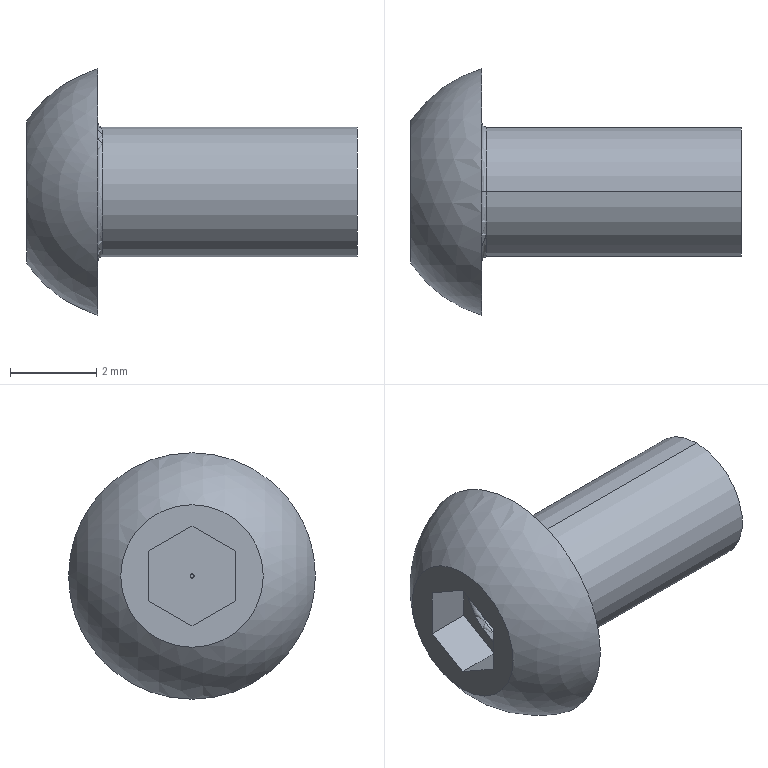Part | NX | features BREP 1 | 1 solid | 21 faces | box 7.65 x 5.7 x 5.7 mm | volume 68.684 mm3 | plane 10 | spline 6 | torus 2 | cylinder 2 | sphere 1 | commonest cylinder face diameters 3 x2
STEP:
#1=CARTESIAN_POINT('',(1.75,0.,1.5));
#2=VERTEX_POINT('',#1);
#3=CARTESIAN_POINT('',(1.75,0.,-1.5));
#4=VERTEX_POINT('',#3);
#5=CARTESIAN_POINT('',(1.75,0.,0.));
#6=DIRECTION('',(1.,0.,0.));
#7=DIRECTION('',(0.,0.,-1.));
#8=AXIS2_PLACEMENT_3D('',#5,#6,#7);
#9=CIRCLE('',#8,1.5);
#10=EDGE_CURVE('',#2,#4,#9,.T.);
#11=ORIENTED_EDGE('',*,*,#10,.F.);
#12=CARTESIAN_POINT('',(1.65,0.,1.6));
#13=VERTEX_POINT('',#12);
#14=CARTESIAN_POINT('',(1.75,0.,1.6));
#15=DIRECTION('',(0.,1.,0.));
#16=DIRECTION('',(0.,0.,1.));
#17=AXIS2_PLACEMENT_3D('',#14,#15,#16);
#18=CIRCLE('',#17,0.1);
#19=EDGE_CURVE('',#13,#2,#18,.F.);
#20=ORIENTED_EDGE('',*,*,#19,.F.);
#21=CARTESIAN_POINT('',(1.65,0.,-1.6));
#22=VERTEX_POINT('',#21);
#23=CARTESIAN_POINT('',(1.65,0.,0.));
#24=DIRECTION('',(-1.,0.,0.));
#25=DIRECTION('',(0.,0.,-1.));
#26=AXIS2_PLACEMENT_3D('',#23,#24,#25);
#27=CIRCLE('',#26,1.6);
#28=EDGE_CURVE('',#22,#13,#27,.T.);
#29=ORIENTED_EDGE('',*,*,#28,.F.);
#30=CARTESIAN_POINT('',(1.75,0.,-1.6));
#31=DIRECTION('',(0.,-1.,0.));
#32=DIRECTION('',(0.,0.,-1.));
#33=AXIS2_PLACEMENT_3D('',#30,#31,#32);
#34=CIRCLE('',#33,0.1);
#35=EDGE_CURVE('',#22,#4,#34,.F.);
#36=ORIENTED_EDGE('',*,*,#35,.T.);
#37=EDGE_LOOP('',(#11,#20,#29,#36));
#38=FACE_BOUND('',#37,.T.);
#39=CARTESIAN_POINT('',(1.75,0.,0.));
#40=DIRECTION('',(1.,0.,0.));
#41=DIRECTION('',(0.,0.,1.));
#42=AXIS2_PLACEMENT_3D('',#39,#40,#41);
#43=TOROIDAL_SURFACE('',#42,1.6,0.1);
#44=ADVANCED_FACE('',(#38),#43,.F.);
#45=CARTESIAN_POINT('',(7.65,0.,1.5));
#46=VERTEX_POINT('',#45);
#47=CARTESIAN_POINT('',(7.65,0.,-1.5));
#48=VERTEX_POINT('',#47);
#49=CARTESIAN_POINT('',(7.65,0.,0.));
#50=DIRECTION('',(-1.,0.,0.));
#51=DIRECTION('',(0.,0.,-1.));
#52=AXIS2_PLACEMENT_3D('',#49,#50,#51);
#53=CIRCLE('',#52,1.5);
#54=EDGE_CURVE('',#46,#48,#53,.T.);
#55=ORIENTED_EDGE('',*,*,#54,.T.);
#56=CARTESIAN_POINT('',(7.65,0.,-1.5));
#57=DIRECTION('',(-1.,0.,0.));
#58=VECTOR('',#57,1000.);
#59=LINE('',#56,#58);
#60=EDGE_CURVE('',#48,#4,#59,.T.);
#61=ORIENTED_EDGE('',*,*,#60,.T.);
#62=CARTESIAN_POINT('',(1.75,0.,0.));
#63=DIRECTION('',(1.,0.,0.));
#64=DIRECTION('',(0.,0.,-1.));
#65=AXIS2_PLACEMENT_3D('',#62,#63,#64);
#66=CIRCLE('',#65,1.5);
#67=EDGE_CURVE('',#4,#2,#66,.T.);
#68=ORIENTED_EDGE('',*,*,#67,.T.);
#69=CARTESIAN_POINT('',(7.65,0.,1.5));
#70=DIRECTION('',(-1.,0.,0.));
#71=VECTOR('',#70,1000.);
#72=LINE('',#69,#71);
#73=EDGE_CURVE('',#46,#2,#72,.T.);
#74=ORIENTED_EDGE('',*,*,#73,.F.);
#75=EDGE_LOOP('',(#55,#61,#68,#74));
#76=FACE_BOUND('',#75,.T.);
#77=CARTESIAN_POINT('',(7.65,0.,0.));
#78=DIRECTION('',(-1.,0.,0.));
#79=DIRECTION('',(0.,0.,-1.));
#80=AXIS2_PLACEMENT_3D('',#77,#78,#79);
#81=CYLINDRICAL_SURFACE('',#80,1.5);
#82=ADVANCED_FACE('',(#76),#81,.T.);
#83=CARTESIAN_POINT('',(1.65,2.85,0.));
#84=VERTEX_POINT('',#83);
#85=CARTESIAN_POINT('',(1.65,-2.85,0.));
#86=VERTEX_POINT('',#85);
#87=CARTESIAN_POINT('',(1.65,0.,0.));
#88=DIRECTION('',(1.,0.,0.));
#89=DIRECTION('',(0.,0.,-1.));
#90=AXIS2_PLACEMENT_3D('',#87,#88,#89);
#91=CIRCLE('',#90,2.85);
#92=EDGE_CURVE('',#84,#86,#91,.T.);
#93=ORIENTED_EDGE('',*,*,#92,.T.);
#94=CARTESIAN_POINT('',(1.65,0.,0.));
#95=DIRECTION('',(1.,0.,0.));
#96=DIRECTION('',(0.,0.,-1.));
#97=AXIS2_PLACEMENT_3D('',#94,#95,#96);
#98=CIRCLE('',#97,2.85);
#99=EDGE_CURVE('',#86,#84,#98,.T.);
#100=ORIENTED_EDGE('',*,*,#99,.T.);
#101=EDGE_LOOP('',(#93,#100));
#102=FACE_BOUND('',#101,.T.);
#103=ORIENTED_EDGE('',*,*,#28,.T.);
#104=CARTESIAN_POINT('',(1.65,0.,0.));
#105=DIRECTION('',(-1.,0.,0.));
#106=DIRECTION('',(0.,0.,-1.));
#107=AXIS2_PLACEMENT_3D('',#104,#105,#106);
#108=CIRCLE('',#107,1.6);
#109=EDGE_CURVE('',#13,#22,#108,.T.);
#110=ORIENTED_EDGE('',*,*,#109,.T.);
#111=EDGE_LOOP('',(#103,#110));
#112=FACE_BOUND('',#111,.T.);
#113=CARTESIAN_POINT('',(1.65,0.,0.));
#114=DIRECTION('',(1.,0.,0.));
#115=DIRECTION('',(0.,-1.,0.));
#116=AXIS2_PLACEMENT_3D('',#113,#114,#115);
#117=PLANE('',#116);
#118=ADVANCED_FACE('',(#102,#112),#117,.T.);
#119=ORIENTED_EDGE('',*,*,#92,.F.);
#120=ORIENTED_EDGE('',*,*,#99,.F.);
#121=EDGE_LOOP('',(#119,#120));
#122=FACE_BOUND('',#121,.T.);
#123=CARTESIAN_POINT('',(0.,1.65,0.));
#124=VERTEX_POINT('',#123);
#125=CARTESIAN_POINT('',(0.,-1.65,0.));
#126=VERTEX_POINT('',#125);
#127=CARTESIAN_POINT('',(0.,0.,0.));
#128=DIRECTION('',(1.,0.,0.));
#129=DIRECTION('',(0.,0.,-1.));
#130=AXIS2_PLACEMENT_3D('',#127,#128,#129);
#131=CIRCLE('',#130,1.65);
#132=EDGE_CURVE('',#124,#126,#131,.T.);
#133=ORIENTED_EDGE('',*,*,#132,.T.);
#134=CARTESIAN_POINT('',(0.,0.,0.));
#135=DIRECTION('',(1.,0.,0.));
#136=DIRECTION('',(0.,0.,-1.));
#137=AXIS2_PLACEMENT_3D('',#134,#135,#136);
#138=CIRCLE('',#137,1.65);
#139=EDGE_CURVE('',#126,#124,#138,.T.);
#140=ORIENTED_EDGE('',*,*,#139,.T.);
#141=EDGE_LOOP('',(#133,#140));
#142=FACE_BOUND('',#141,.T.);
#143=CARTESIAN_POINT('',(2.461,0.,0.));
#144=DIRECTION('',(0.,1.,0.));
#145=DIRECTION('',(-0.2585,0.,-0.966));
#146=AXIS2_PLACEMENT_3D('',#143,#144,#145);
#147=SPHERICAL_SURFACE('',#146,2.963);
#148=ADVANCED_FACE('',(#122,#142),#147,.T.);
#149=ORIENTED_EDGE('',*,*,#132,.F.);
#150=ORIENTED_EDGE('',*,*,#139,.F.);
#151=EDGE_LOOP('',(#149,#150));
#152=FACE_BOUND('',#151,.T.);
#153=CARTESIAN_POINT('',(0.,1.,-0.5774));
#154=VERTEX_POINT('',#153);
#155=CARTESIAN_POINT('',(0.,0.,-1.155));
#156=VERTEX_POINT('',#155);
#157=CARTESIAN_POINT('',(0.,1.,-0.5774));
#158=DIRECTION('',(0.,-0.866,-0.5));
#159=VECTOR('',#158,1000.);
#160=LINE('',#157,#159);
#161=EDGE_CURVE('',#154,#156,#160,.T.);
#162=ORIENTED_EDGE('',*,*,#161,.F.);
#163=CARTESIAN_POINT('',(0.,1.,0.5774));
#164=VERTEX_POINT('',#163);
#165=CARTESIAN_POINT('',(0.,1.,0.));
#166=DIRECTION('',(0.,0.,-1.));
#167=VECTOR('',#166,1000.);
#168=LINE('',#165,#167);
#169=EDGE_CURVE('',#164,#154,#168,.T.);
#170=ORIENTED_EDGE('',*,*,#169,.F.);
#171=CARTESIAN_POINT('',(0.,0.,1.155));
#172=VERTEX_POINT('',#171);
#173=CARTESIAN_POINT('',(0.,0.,1.155));
#174=DIRECTION('',(0.,0.866,-0.5));
#175=VECTOR('',#174,1000.);
#176=LINE('',#173,#175);
#177=EDGE_CURVE('',#172,#164,#176,.T.);
#178=ORIENTED_EDGE('',*,*,#177,.F.);
#179=CARTESIAN_POINT('',(0.,-1.,0.5774));
#180=VERTEX_POINT('',#179);
#181=CARTESIAN_POINT('',(0.,-1.,0.5774));
#182=DIRECTION('',(0.,0.866,0.5));
#183=VECTOR('',#182,1000.);
#184=LINE('',#181,#183);
#185=EDGE_CURVE('',#180,#172,#184,.T.);
#186=ORIENTED_EDGE('',*,*,#185,.F.);
#187=CARTESIAN_POINT('',(0.,-1.,-0.5774));
#188=VERTEX_POINT('',#187);
#189=CARTESIAN_POINT('',(0.,-1.,0.));
#190=DIRECTION('',(0.,0.,1.));
#191=VECTOR('',#190,1000.);
#192=LINE('',#189,#191);
#193=EDGE_CURVE('',#188,#180,#192,.T.);
#194=ORIENTED_EDGE('',*,*,#193,.F.);
#195=CARTESIAN_POINT('',(0.,0.,-1.155));
#196=DIRECTION('',(0.,-0.866,0.5));
#197=VECTOR('',#196,1000.);
#198=LINE('',#195,#197);
#199=EDGE_CURVE('',#156,#188,#198,.T.);
#200=ORIENTED_EDGE('',*,*,#199,.F.);
#201=EDGE_LOOP('',(#162,#170,#178,#186,#194,#200));
#202=FACE_BOUND('',#201,.T.);
#203=CARTESIAN_POINT('',(0.,0.,0.));
#204=DIRECTION('',(1.,0.,0.));
#205=DIRECTION('',(0.,-1.,0.));
#206=AXIS2_PLACEMENT_3D('',#203,#204,#205);
#207=PLANE('',#206);
#208=ADVANCED_FACE('',(#152,#202),#207,.F.);
#209=CARTESIAN_POINT('',(1.04,-1.,-0.5774));
#210=VERTEX_POINT('',#209);
#211=CARTESIAN_POINT('',(1.04,0.,-1.155));
#212=VERTEX_POINT('',#211);
#213=CARTESIAN_POINT('',(1.04,-1.,-0.5774));
#214=DIRECTION('',(0.,0.866,-0.5));
#215=VECTOR('',#214,1000.);
#216=LINE('',#213,#215);
#217=EDGE_CURVE('',#210,#212,#216,.T.);
#218=ORIENTED_EDGE('',*,*,#217,.T.);
#219=CARTESIAN_POINT('',(1.04,0.,-1.155));
#220=DIRECTION('',(-1.,0.,0.));
#221=VECTOR('',#220,1000.);
#222=LINE('',#219,#221);
#223=EDGE_CURVE('',#212,#156,#222,.T.);
#224=ORIENTED_EDGE('',*,*,#223,.T.);
#225=ORIENTED_EDGE('',*,*,#199,.T.);
#226=CARTESIAN_POINT('',(1.04,-1.,-0.5774));
#227=DIRECTION('',(1.,0.,0.));
#228=VECTOR('',#227,1000.);
#229=LINE('',#226,#228);
#230=EDGE_CURVE('',#188,#210,#229,.T.);
#231=ORIENTED_EDGE('',*,*,#230,.T.);
#232=EDGE_LOOP('',(#218,#224,#225,#231));
#233=FACE_BOUND('',#232,.T.);
#234=CARTESIAN_POINT('',(1.04,-1.,-0.5774));
#235=DIRECTION('',(0.,0.5,0.866));
#236=DIRECTION('',(-1.,0.,0.));
#237=AXIS2_PLACEMENT_3D('',#234,#235,#236);
#238=PLANE('',#237);
#239=ADVANCED_FACE('',(#233),#238,.T.);
#240=CARTESIAN_POINT('',(1.04,1.,-0.5774));
#241=VERTEX_POINT('',#240);
#242=CARTESIAN_POINT('',(1.04,0.,-1.155));
#243=DIRECTION('',(0.,0.866,0.5));
#244=VECTOR('',#243,1000.);
#245=LINE('',#242,#244);
#246=EDGE_CURVE('',#212,#241,#245,.T.);
#247=ORIENTED_EDGE('',*,*,#246,.T.);
#248=CARTESIAN_POINT('',(1.04,1.,-0.5774));
#249=DIRECTION('',(-1.,0.,0.));
#250=VECTOR('',#249,1000.);
#251=LINE('',#248,#250);
#252=EDGE_CURVE('',#241,#154,#251,.T.);
#253=ORIENTED_EDGE('',*,*,#252,.T.);
#254=ORIENTED_EDGE('',*,*,#161,.T.);
#255=ORIENTED_EDGE('',*,*,#223,.F.);
#256=EDGE_LOOP('',(#247,#253,#254,#255));
#257=FACE_BOUND('',#256,.T.);
#258=CARTESIAN_POINT('',(1.04,0.,-1.155));
#259=DIRECTION('',(0.,-0.5,0.866));
#260=DIRECTION('',(1.,0.,0.));
#261=AXIS2_PLACEMENT_3D('',#258,#259,#260);
#262=PLANE('',#261);
#263=ADVANCED_FACE('',(#257),#262,.T.);
#264=CARTESIAN_POINT('',(1.04,1.,0.5774));
#265=VERTEX_POINT('',#264);
#266=CARTESIAN_POINT('',(1.04,1.,-0.5774));
#267=DIRECTION('',(0.,0.,1.));
#268=VECTOR('',#267,1000.);
#269=LINE('',#266,#268);
#270=EDGE_CURVE('',#241,#265,#269,.T.);
#271=ORIENTED_EDGE('',*,*,#270,.T.);
#272=CARTESIAN_POINT('',(1.04,1.,0.5774));
#273=DIRECTION('',(-1.,0.,0.));
#274=VECTOR('',#273,1000.);
#275=LINE('',#272,#274);
#276=EDGE_CURVE('',#265,#164,#275,.T.);
#277=ORIENTED_EDGE('',*,*,#276,.T.);
#278=ORIENTED_EDGE('',*,*,#169,.T.);
#279=ORIENTED_EDGE('',*,*,#252,.F.);
#280=EDGE_LOOP('',(#271,#277,#278,#279));
#281=FACE_BOUND('',#280,.T.);
#282=CARTESIAN_POINT('',(1.04,1.,-0.5774));
#283=DIRECTION('',(0.,-1.,0.));
#284=DIRECTION('',(1.,0.,0.));
#285=AXIS2_PLACEMENT_3D('',#282,#283,#284);
#286=PLANE('',#285);
#287=ADVANCED_FACE('',(#281),#286,.T.);
#288=CARTESIAN_POINT('',(1.04,0.,1.155));
#289=VERTEX_POINT('',#288);
#290=CARTESIAN_POINT('',(1.04,1.,0.5774));
#291=DIRECTION('',(0.,-0.866,0.5));
#292=VECTOR('',#291,1000.);
#293=LINE('',#290,#292);
#294=EDGE_CURVE('',#265,#289,#293,.T.);
#295=ORIENTED_EDGE('',*,*,#294,.T.);
#296=CARTESIAN_POINT('',(1.04,0.,1.155));
#297=DIRECTION('',(-1.,0.,0.));
#298=VECTOR('',#297,1000.);
#299=LINE('',#296,#298);
#300=EDGE_CURVE('',#289,#172,#299,.T.);
#301=ORIENTED_EDGE('',*,*,#300,.T.);
#302=ORIENTED_EDGE('',*,*,#177,.T.);
#303=ORIENTED_EDGE('',*,*,#276,.F.);
#304=EDGE_LOOP('',(#295,#301,#302,#303));
#305=FACE_BOUND('',#304,.T.);
#306=CARTESIAN_POINT('',(1.04,1.,0.5774));
#307=DIRECTION('',(0.,-0.5,-0.866));
#308=DIRECTION('',(0.,0.866,-0.5));
#309=AXIS2_PLACEMENT_3D('',#306,#307,#308);
#310=PLANE('',#309);
#311=ADVANCED_FACE('',(#305),#310,.T.);
#312=CARTESIAN_POINT('',(1.04,-1.,0.5774));
#313=VERTEX_POINT('',#312);
#314=CARTESIAN_POINT('',(1.04,0.,1.155));
#315=DIRECTION('',(0.,-0.866,-0.5));
#316=VECTOR('',#315,1000.);
#317=LINE('',#314,#316);
#318=EDGE_CURVE('',#289,#313,#317,.T.);
#319=ORIENTED_EDGE('',*,*,#318,.T.);
#320=CARTESIAN_POINT('',(1.04,-1.,0.5774));
#321=DIRECTION('',(-1.,0.,0.));
#322=VECTOR('',#321,1000.);
#323=LINE('',#320,#322);
#324=EDGE_CURVE('',#313,#180,#323,.T.);
#325=ORIENTED_EDGE('',*,*,#324,.T.);
#326=ORIENTED_EDGE('',*,*,#185,.T.);
#327=ORIENTED_EDGE('',*,*,#300,.F.);
#328=EDGE_LOOP('',(#319,#325,#326,#327));
#329=FACE_BOUND('',#328,.T.);
#330=CARTESIAN_POINT('',(1.04,0.,1.155));
#331=DIRECTION('',(0.,0.5,-0.866));
#332=DIRECTION('',(1.,0.,0.));
#333=AXIS2_PLACEMENT_3D('',#330,#331,#332);
#334=PLANE('',#333);
#335=ADVANCED_FACE('',(#329),#334,.T.);
#336=CARTESIAN_POINT('',(1.04,-1.,0.5774));
#337=DIRECTION('',(0.,0.,-1.));
#338=VECTOR('',#337,1000.);
#339=LINE('',#336,#338);
#340=EDGE_CURVE('',#313,#210,#339,.T.);
#341=ORIENTED_EDGE('',*,*,#340,.T.);
#342=ORIENTED_EDGE('',*,*,#230,.F.);
#343=ORIENTED_EDGE('',*,*,#193,.T.);
#344=ORIENTED_EDGE('',*,*,#324,.F.);
#345=EDGE_LOOP('',(#341,#342,#343,#344));
#346=FACE_BOUND('',#345,.T.);
#347=CARTESIAN_POINT('',(1.04,-1.,0.5774));
#348=DIRECTION('',(0.,1.,0.));
#349=DIRECTION('',(-1.,0.,0.));
#350=AXIS2_PLACEMENT_3D('',#347,#348,#349);
#351=PLANE('',#350);
#352=ADVANCED_FACE('',(#346),#351,.T.);
#353=CARTESIAN_POINT('',(1.542,-0.022,-0.0381));
#354=VERTEX_POINT('',#353);
#355=CARTESIAN_POINT('',(1.04,-1.,-0.5774));
#356=CARTESIAN_POINT('',(1.121,-0.845,-0.4878));
#357=CARTESIAN_POINT('',(1.204,-0.6803,-0.3988));
#358=CARTESIAN_POINT('',(1.372,-0.3525,-0.2177));
#359=CARTESIAN_POINT('',(1.399,-0.3014,-0.1869));
#360=CARTESIAN_POINT('',(1.526,-0.0494,-0.05698));
#361=CARTESIAN_POINT('',(1.541,-0.0292,-0.03808));
#362=CARTESIAN_POINT('',(1.543,-0.02217,-0.0384));
#363=B_SPLINE_CURVE_WITH_KNOTS('',3,(#355,#356,#357,#358,#359,#360,#361,#362),.UNSPECIFIED.,.F.,.F.,(4,1,1,1,1,4),(0.,0.5,0.625,0.75,0.875,1.),.UNSPECIFIED.);
#364=EDGE_CURVE('',#354,#210,#363,.F.);
#365=ORIENTED_EDGE('',*,*,#364,.F.);
#366=CARTESIAN_POINT('',(1.543,-0.02217,-0.0384));
#367=CARTESIAN_POINT('',(1.546,-0.01126,-0.03849));
#368=CARTESIAN_POINT('',(1.469,-0.02,-0.1962));
#369=CARTESIAN_POINT('',(1.414,-0.01237,-0.3217));
#370=CARTESIAN_POINT('',(1.369,-0.01206,-0.4203));
#371=CARTESIAN_POINT('',(1.257,-0.007308,-0.6718));
#372=CARTESIAN_POINT('',(1.2,-0.005747,-0.7972));
#373=CARTESIAN_POINT('',(1.095,-0.001899,-1.032));
#374=CARTESIAN_POINT('',(1.04,0.,-1.155));
#375=B_SPLINE_CURVE_WITH_KNOTS('',3,(#366,#367,#368,#369,#370,#371,#372,#373,#374),.UNSPECIFIED.,.F.,.F.,(4,1,1,1,1,1,4),(0.,0.125,0.25,0.375,0.5,0.75,1.),.UNSPECIFIED.);
#376=EDGE_CURVE('',#212,#354,#375,.F.);
#377=ORIENTED_EDGE('',*,*,#376,.F.);
#378=ORIENTED_EDGE('',*,*,#217,.F.);
#379=EDGE_LOOP('',(#365,#377,#378));
#380=FACE_BOUND('',#379,.T.);
#381=CARTESIAN_POINT('',(1.04,-1.,-0.5774));
#382=CARTESIAN_POINT('',(1.207,-0.6811,-0.3932));
#383=CARTESIAN_POINT('',(1.373,-0.3622,-0.2091));
#384=CARTESIAN_POINT('',(1.542,-0.04011,-0.02316));
#385=CARTESIAN_POINT('',(1.543,-0.03692,-0.02132));
#386=CARTESIAN_POINT('',(1.545,-0.03373,-0.01948));
#387=CARTESIAN_POINT('',(1.04,-0.8333,-0.6736));
#388=CARTESIAN_POINT('',(1.207,-0.5686,-0.4598));
#389=CARTESIAN_POINT('',(1.373,-0.3039,-0.246));
#390=CARTESIAN_POINT('',(1.542,-0.03649,-0.03008));
#391=CARTESIAN_POINT('',(1.543,-0.03384,-0.02794));
#392=CARTESIAN_POINT('',(1.545,-0.03119,-0.0258));
#393=CARTESIAN_POINT('',(1.04,-0.6667,-0.7698));
#394=CARTESIAN_POINT('',(1.207,-0.4553,-0.526));
#395=CARTESIAN_POINT('',(1.373,-0.2439,-0.2822));
#396=CARTESIAN_POINT('',(1.542,-0.03036,-0.03603));
#397=CARTESIAN_POINT('',(1.543,-0.02825,-0.03359));
#398=CARTESIAN_POINT('',(1.545,-0.02613,-0.03115));
#399=CARTESIAN_POINT('',(1.04,-0.3333,-0.9623));
#400=CARTESIAN_POINT('',(1.207,-0.2279,-0.6573));
#401=CARTESIAN_POINT('',(1.373,-0.1225,-0.3523));
#402=CARTESIAN_POINT('',(1.542,-0.01602,-0.04431));
#403=CARTESIAN_POINT('',(1.543,-0.01497,-0.04126));
#404=CARTESIAN_POINT('',(1.545,-0.01391,-0.03821));
#405=CARTESIAN_POINT('',(1.04,-0.1667,-1.058));
#406=CARTESIAN_POINT('',(1.207,-0.1139,-0.7223));
#407=CARTESIAN_POINT('',(1.373,-0.06111,-0.3862));
#408=CARTESIAN_POINT('',(1.542,-0.007806,-0.04664));
#409=CARTESIAN_POINT('',(1.543,-0.007278,-0.04328));
#410=CARTESIAN_POINT('',(1.545,-0.00675,-0.03992));
#411=CARTESIAN_POINT('',(1.04,0.,-1.155));
#412=CARTESIAN_POINT('',(1.207,0.,-0.7865));
#413=CARTESIAN_POINT('',(1.373,0.,-0.4182));
#414=CARTESIAN_POINT('',(1.542,0.,-0.04632));
#415=CARTESIAN_POINT('',(1.543,0.,-0.04264));
#416=CARTESIAN_POINT('',(1.545,0.,-0.03895));
#417=B_SPLINE_SURFACE_WITH_KNOTS('',3,3,((#381,#382,#383,#384,#385,#386),(#387,#388,#389,#390,#391,#392),(#393,#394,#395,#396,#397,#398),(#399,#400,#401,#402,#403,#404),(#405,#406,#407,#408,#409,#410),(#411,#412,#413,#414,#415,#416)),.RULED_SURF.,.F.,.F.,.F.,(4,2,4),(4,2,4),(0.,0.5,1.),(0.,0.9901,1.),.UNSPECIFIED.);
#418=ADVANCED_FACE('',(#380),#417,.F.);
#419=ORIENTED_EDGE('',*,*,#376,.T.);
#420=CARTESIAN_POINT('',(1.542,0.04399,0.));
#421=VERTEX_POINT('',#420);
#422=CARTESIAN_POINT('',(1.54,0.04399,0.));
#423=CARTESIAN_POINT('',(1.54,0.05112,-0.03859));
#424=CARTESIAN_POINT('',(1.54,0.008464,-0.06403));
#425=CARTESIAN_POINT('',(1.54,-0.022,-0.0381));
#426=B_SPLINE_CURVE_WITH_KNOTS('',3,(#422,#423,#424,#425),.UNSPECIFIED.,.F.,.F.,(4,4),(0.,1.),.UNSPECIFIED.);
#427=EDGE_CURVE('',#421,#354,#426,.T.);
#428=ORIENTED_EDGE('',*,*,#427,.F.);
#429=CARTESIAN_POINT('',(1.544,0.04448,-0.0005402));
#430=CARTESIAN_POINT('',(1.543,0.04731,-0.00108));
#431=CARTESIAN_POINT('',(1.528,0.0899,-0.02055));
#432=CARTESIAN_POINT('',(1.432,0.2651,-0.1353));
#433=CARTESIAN_POINT('',(1.403,0.3189,-0.1671));
#434=CARTESIAN_POINT('',(1.278,0.5543,-0.3097));
#435=CARTESIAN_POINT('',(1.253,0.6008,-0.3374));
#436=CARTESIAN_POINT('',(1.167,0.7617,-0.4341));
#437=CARTESIAN_POINT('',(1.096,0.8947,-0.5141));
#438=CARTESIAN_POINT('',(1.04,1.,-0.5774));
#439=B_SPLINE_CURVE_WITH_KNOTS('',3,(#429,#430,#431,#432,#433,#434,#435,#436,#437,#438),.UNSPECIFIED.,.F.,.F.,(4,1,1,1,1,1,1,4),(0.,0.125,0.25,0.375,0.5,0.625,0.75,1.),.UNSPECIFIED.);
#440=EDGE_CURVE('',#241,#421,#439,.F.);
#441=ORIENTED_EDGE('',*,*,#440,.F.);
#442=ORIENTED_EDGE('',*,*,#246,.F.);
#443=EDGE_LOOP('',(#419,#428,#441,#442));
#444=FACE_BOUND('',#443,.T.);
#445=CARTESIAN_POINT('',(1.04,-0.5135,-1.451));
#446=CARTESIAN_POINT('',(1.207,-0.3509,-0.9841));
#447=CARTESIAN_POINT('',(1.373,-0.1883,-0.5171));
#448=CARTESIAN_POINT('',(1.542,-0.02405,-0.04533));
#449=CARTESIAN_POINT('',(1.543,-0.02242,-0.04066));
#450=CARTESIAN_POINT('',(1.545,-0.0208,-0.03599));
#451=CARTESIAN_POINT('',(1.04,-0.3423,-1.352));
#452=CARTESIAN_POINT('',(1.207,-0.2339,-0.9182));
#453=CARTESIAN_POINT('',(1.373,-0.1255,-0.4841));
#454=CARTESIAN_POINT('',(1.542,-0.01603,-0.04566));
#455=CARTESIAN_POINT('',(1.543,-0.01495,-0.04132));
#456=CARTESIAN_POINT('',(1.545,-0.01386,-0.03698));
#457=CARTESIAN_POINT('',(1.04,-0.1712,-1.254));
#458=CARTESIAN_POINT('',(1.207,-0.117,-0.8523));
#459=CARTESIAN_POINT('',(1.373,-0.06276,-0.4512));
#460=CARTESIAN_POINT('',(1.542,-0.008016,-0.04599));
#461=CARTESIAN_POINT('',(1.543,-0.007474,-0.04198));
#462=CARTESIAN_POINT('',(1.545,-0.006932,-0.03796));
#463=CARTESIAN_POINT('',(1.04,0.1667,-1.058));
#464=CARTESIAN_POINT('',(1.207,0.1139,-0.7223));
#465=CARTESIAN_POINT('',(1.373,0.06111,-0.3862));
#466=CARTESIAN_POINT('',(1.542,0.007806,-0.04664));
#467=CARTESIAN_POINT('',(1.543,0.007278,-0.04328));
#468=CARTESIAN_POINT('',(1.545,0.00675,-0.03992));
#469=CARTESIAN_POINT('',(1.04,0.3333,-0.9623));
#470=CARTESIAN_POINT('',(1.207,0.2279,-0.6573));
#471=CARTESIAN_POINT('',(1.373,0.1225,-0.3523));
#472=CARTESIAN_POINT('',(1.542,0.01602,-0.04431));
#473=CARTESIAN_POINT('',(1.543,0.01497,-0.04126));
#474=CARTESIAN_POINT('',(1.545,0.01391,-0.03821));
#475=CARTESIAN_POINT('',(1.04,0.6667,-0.7698));
#476=CARTESIAN_POINT('',(1.207,0.4553,-0.526));
#477=CARTESIAN_POINT('',(1.373,0.2439,-0.2822));
#478=CARTESIAN_POINT('',(1.542,0.03036,-0.03603));
#479=CARTESIAN_POINT('',(1.543,0.02825,-0.03359));
#480=CARTESIAN_POINT('',(1.545,0.02613,-0.03115));
#481=CARTESIAN_POINT('',(1.04,0.8333,-0.6736));
#482=CARTESIAN_POINT('',(1.207,0.5686,-0.4598));
#483=CARTESIAN_POINT('',(1.373,0.3039,-0.246));
#484=CARTESIAN_POINT('',(1.542,0.03649,-0.03008));
#485=CARTESIAN_POINT('',(1.543,0.03384,-0.02794));
#486=CARTESIAN_POINT('',(1.545,0.03119,-0.0258));
#487=CARTESIAN_POINT('',(1.04,1.171,-0.4785));
#488=CARTESIAN_POINT('',(1.207,0.7966,-0.3249));
#489=CARTESIAN_POINT('',(1.373,0.4221,-0.1712));
#490=CARTESIAN_POINT('',(1.542,0.04384,-0.01605));
#491=CARTESIAN_POINT('',(1.543,0.04009,-0.01452));
#492=CARTESIAN_POINT('',(1.545,0.03634,-0.01298));
#493=CARTESIAN_POINT('',(1.04,1.342,-0.3797));
#494=CARTESIAN_POINT('',(1.207,0.9122,-0.2565));
#495=CARTESIAN_POINT('',(1.373,0.482,-0.1334));
#496=CARTESIAN_POINT('',(1.542,0.04756,-0.008945));
#497=CARTESIAN_POINT('',(1.543,0.04326,-0.007713));
#498=CARTESIAN_POINT('',(1.545,0.03895,-0.006482));
#499=CARTESIAN_POINT('',(1.04,1.513,-0.2809));
#500=CARTESIAN_POINT('',(1.207,1.028,-0.1882));
#501=CARTESIAN_POINT('',(1.373,0.5419,-0.09547));
#502=CARTESIAN_POINT('',(1.542,0.05128,-0.001838));
#503=CARTESIAN_POINT('',(1.543,0.04642,-0.0009111));
#504=CARTESIAN_POINT('',(1.545,0.04156,0.00001596));
#505=B_SPLINE_SURFACE_WITH_KNOTS('',3,3,((#445,#446,#447,#448,#449,#450),(#451,#452,#453,#454,#455,#456),(#457,#458,#459,#460,#461,#462),(#463,#464,#465,#466,#467,#468),(#469,#470,#471,#472,#473,#474),(#475,#476,#477,#478,#479,#480),(#481,#482,#483,#484,#485,#486),(#487,#488,#489,#490,#491,#492),(#493,#494,#495,#496,#497,#498),(#499,#500,#501,#502,#503,#504)),.RULED_SURF.,.F.,.F.,.F.,(4,2,2,2,4),(4,2,4),(0.,0.2533,0.5,0.7467,1.),(0.,0.9901,1.),.UNSPECIFIED.);
#506=ADVANCED_FACE('',(#444),#505,.F.);
#507=ORIENTED_EDGE('',*,*,#440,.T.);
#508=CARTESIAN_POINT('',(1.543,0.04434,0.));
#509=CARTESIAN_POINT('',(1.546,0.03897,0.009492));
#510=CARTESIAN_POINT('',(1.469,0.1799,0.08079));
#511=CARTESIAN_POINT('',(1.414,0.2848,0.1501));
#512=CARTESIAN_POINT('',(1.369,0.3701,0.1997));
#513=CARTESIAN_POINT('',(1.257,0.5855,0.3296));
#514=CARTESIAN_POINT('',(1.2,0.6932,0.3936));
#515=CARTESIAN_POINT('',(1.095,0.8945,0.5143));
#516=CARTESIAN_POINT('',(1.04,1.,0.5774));
#517=B_SPLINE_CURVE_WITH_KNOTS('',3,(#508,#509,#510,#511,#512,#513,#514,#515,#516),.UNSPECIFIED.,.F.,.F.,(4,1,1,1,1,1,4),(0.,0.125,0.25,0.375,0.5,0.75,1.),.UNSPECIFIED.);
#518=EDGE_CURVE('',#265,#421,#517,.F.);
#519=ORIENTED_EDGE('',*,*,#518,.F.);
#520=ORIENTED_EDGE('',*,*,#270,.F.);
#521=EDGE_LOOP('',(#507,#519,#520));
#522=FACE_BOUND('',#521,.T.);
#523=CARTESIAN_POINT('',(1.04,1.,-0.5774));
#524=CARTESIAN_POINT('',(1.207,0.6811,-0.3932));
#525=CARTESIAN_POINT('',(1.373,0.3622,-0.2091));
#526=CARTESIAN_POINT('',(1.542,0.04011,-0.02316));
#527=CARTESIAN_POINT('',(1.543,0.03692,-0.02132));
#528=CARTESIAN_POINT('',(1.545,0.03373,-0.01948));
#529=CARTESIAN_POINT('',(1.04,1.,-0.3849));
#530=CARTESIAN_POINT('',(1.207,0.6825,-0.2625));
#531=CARTESIAN_POINT('',(1.373,0.365,-0.1402));
#532=CARTESIAN_POINT('',(1.542,0.04429,-0.01656));
#533=CARTESIAN_POINT('',(1.543,0.04112,-0.01534));
#534=CARTESIAN_POINT('',(1.545,0.03794,-0.01411));
#535=CARTESIAN_POINT('',(1.04,1.,-0.1925));
#536=CARTESIAN_POINT('',(1.207,0.6832,-0.1313));
#537=CARTESIAN_POINT('',(1.373,0.3664,-0.07008));
#538=CARTESIAN_POINT('',(1.542,0.04638,-0.00828));
#539=CARTESIAN_POINT('',(1.543,0.04321,-0.007668));
#540=CARTESIAN_POINT('',(1.545,0.04005,-0.007056));
#541=CARTESIAN_POINT('',(1.04,1.,0.1925));
#542=CARTESIAN_POINT('',(1.207,0.6832,0.1313));
#543=CARTESIAN_POINT('',(1.373,0.3664,0.07008));
#544=CARTESIAN_POINT('',(1.542,0.04638,0.00828));
#545=CARTESIAN_POINT('',(1.543,0.04321,0.007668));
#546=CARTESIAN_POINT('',(1.545,0.04005,0.007056));
#547=CARTESIAN_POINT('',(1.04,1.,0.3849));
#548=CARTESIAN_POINT('',(1.207,0.6825,0.2625));
#549=CARTESIAN_POINT('',(1.373,0.365,0.1402));
#550=CARTESIAN_POINT('',(1.542,0.04429,0.01656));
#551=CARTESIAN_POINT('',(1.543,0.04112,0.01534));
#552=CARTESIAN_POINT('',(1.545,0.03794,0.01411));
#553=CARTESIAN_POINT('',(1.04,1.,0.5774));
#554=CARTESIAN_POINT('',(1.207,0.6811,0.3932));
#555=CARTESIAN_POINT('',(1.373,0.3622,0.2091));
#556=CARTESIAN_POINT('',(1.542,0.04011,0.02316));
#557=CARTESIAN_POINT('',(1.543,0.03692,0.02132));
#558=CARTESIAN_POINT('',(1.545,0.03373,0.01948));
#559=B_SPLINE_SURFACE_WITH_KNOTS('',3,3,((#523,#524,#525,#526,#527,#528),(#529,#530,#531,#532,#533,#534),(#535,#536,#537,#538,#539,#540),(#541,#542,#543,#544,#545,#546),(#547,#548,#549,#550,#551,#552),(#553,#554,#555,#556,#557,#558)),.RULED_SURF.,.F.,.F.,.F.,(4,2,4),(4,2,4),(0.,0.5,1.),(0.,0.9901,1.),.UNSPECIFIED.);
#560=ADVANCED_FACE('',(#522),#559,.F.);
#561=ORIENTED_EDGE('',*,*,#518,.T.);
#562=CARTESIAN_POINT('',(1.542,-0.022,0.0381));
#563=VERTEX_POINT('',#562);
#564=CARTESIAN_POINT('',(1.54,-0.022,0.0381));
#565=CARTESIAN_POINT('',(1.54,0.007863,0.06357));
#566=CARTESIAN_POINT('',(1.54,0.05122,0.03935));
#567=CARTESIAN_POINT('',(1.54,0.04399,0.));
#568=B_SPLINE_CURVE_WITH_KNOTS('',3,(#564,#565,#566,#567),.UNSPECIFIED.,.F.,.F.,(4,4),(0.,1.),.UNSPECIFIED.);
#569=EDGE_CURVE('',#563,#421,#568,.T.);
#570=ORIENTED_EDGE('',*,*,#569,.F.);
#571=CARTESIAN_POINT('',(1.544,-0.02177,0.03879));
#572=CARTESIAN_POINT('',(1.543,-0.02272,0.04151));
#573=CARTESIAN_POINT('',(1.528,-0.02716,0.08813));
#574=CARTESIAN_POINT('',(1.432,-0.01539,0.2973));
#575=CARTESIAN_POINT('',(1.403,-0.01471,0.3598));
#576=CARTESIAN_POINT('',(1.278,-0.008951,0.6349));
#577=CARTESIAN_POINT('',(1.253,-0.008241,0.689));
#578=CARTESIAN_POINT('',(1.167,-0.004903,0.8767));
#579=CARTESIAN_POINT('',(1.096,-0.002132,1.032));
#580=CARTESIAN_POINT('',(1.04,0.,1.155));
#581=B_SPLINE_CURVE_WITH_KNOTS('',3,(#571,#572,#573,#574,#575,#576,#577,#578,#579,#580),.UNSPECIFIED.,.F.,.F.,(4,1,1,1,1,1,1,4),(0.,0.125,0.25,0.375,0.5,0.625,0.75,1.),.UNSPECIFIED.);
#582=EDGE_CURVE('',#289,#563,#581,.F.);
#583=ORIENTED_EDGE('',*,*,#582,.F.);
#584=ORIENTED_EDGE('',*,*,#294,.F.);
#585=EDGE_LOOP('',(#561,#570,#583,#584));
#586=FACE_BOUND('',#585,.T.);
#587=CARTESIAN_POINT('',(1.04,1.513,0.2809));
#588=CARTESIAN_POINT('',(1.207,1.028,0.1882));
#589=CARTESIAN_POINT('',(1.373,0.5419,0.09547));
#590=CARTESIAN_POINT('',(1.542,0.05128,0.001838));
#591=CARTESIAN_POINT('',(1.543,0.04642,0.0009111));
#592=CARTESIAN_POINT('',(1.545,0.04156,-0.00001596));
#593=CARTESIAN_POINT('',(1.04,1.342,0.3797));
#594=CARTESIAN_POINT('',(1.207,0.9122,0.2565));
#595=CARTESIAN_POINT('',(1.373,0.482,0.1334));
#596=CARTESIAN_POINT('',(1.542,0.04756,0.008945));
#597=CARTESIAN_POINT('',(1.543,0.04326,0.007713));
#598=CARTESIAN_POINT('',(1.545,0.03895,0.006482));
#599=CARTESIAN_POINT('',(1.04,1.171,0.4785));
#600=CARTESIAN_POINT('',(1.207,0.7966,0.3249));
#601=CARTESIAN_POINT('',(1.373,0.4221,0.1712));
#602=CARTESIAN_POINT('',(1.542,0.04384,0.01605));
#603=CARTESIAN_POINT('',(1.543,0.04009,0.01452));
#604=CARTESIAN_POINT('',(1.545,0.03634,0.01298));
#605=CARTESIAN_POINT('',(1.04,0.8333,0.6736));
#606=CARTESIAN_POINT('',(1.207,0.5686,0.4598));
#607=CARTESIAN_POINT('',(1.373,0.3039,0.246));
#608=CARTESIAN_POINT('',(1.542,0.03649,0.03008));
#609=CARTESIAN_POINT('',(1.543,0.03384,0.02794));
#610=CARTESIAN_POINT('',(1.545,0.03119,0.0258));
#611=CARTESIAN_POINT('',(1.04,0.6667,0.7698));
#612=CARTESIAN_POINT('',(1.207,0.4553,0.526));
#613=CARTESIAN_POINT('',(1.373,0.2439,0.2822));
#614=CARTESIAN_POINT('',(1.542,0.03036,0.03603));
#615=CARTESIAN_POINT('',(1.543,0.02825,0.03359));
#616=CARTESIAN_POINT('',(1.545,0.02613,0.03115));
#617=CARTESIAN_POINT('',(1.04,0.3333,0.9623));
#618=CARTESIAN_POINT('',(1.207,0.2279,0.6573));
#619=CARTESIAN_POINT('',(1.373,0.1225,0.3523));
#620=CARTESIAN_POINT('',(1.542,0.01602,0.04431));
#621=CARTESIAN_POINT('',(1.543,0.01497,0.04126));
#622=CARTESIAN_POINT('',(1.545,0.01391,0.03821));
#623=CARTESIAN_POINT('',(1.04,0.1667,1.058));
#624=CARTESIAN_POINT('',(1.207,0.1139,0.7223));
#625=CARTESIAN_POINT('',(1.373,0.06111,0.3862));
#626=CARTESIAN_POINT('',(1.542,0.007806,0.04664));
#627=CARTESIAN_POINT('',(1.543,0.007278,0.04328));
#628=CARTESIAN_POINT('',(1.545,0.00675,0.03992));
#629=CARTESIAN_POINT('',(1.04,-0.1712,1.254));
#630=CARTESIAN_POINT('',(1.207,-0.117,0.8523));
#631=CARTESIAN_POINT('',(1.373,-0.06276,0.4512));
#632=CARTESIAN_POINT('',(1.542,-0.008016,0.04599));
#633=CARTESIAN_POINT('',(1.543,-0.007474,0.04198));
#634=CARTESIAN_POINT('',(1.545,-0.006932,0.03796));
#635=CARTESIAN_POINT('',(1.04,-0.3423,1.352));
#636=CARTESIAN_POINT('',(1.207,-0.2339,0.9182));
#637=CARTESIAN_POINT('',(1.373,-0.1255,0.4841));
#638=CARTESIAN_POINT('',(1.542,-0.01603,0.04566));
#639=CARTESIAN_POINT('',(1.543,-0.01495,0.04132));
#640=CARTESIAN_POINT('',(1.545,-0.01386,0.03698));
#641=CARTESIAN_POINT('',(1.04,-0.5135,1.451));
#642=CARTESIAN_POINT('',(1.207,-0.3509,0.9841));
#643=CARTESIAN_POINT('',(1.373,-0.1883,0.5171));
#644=CARTESIAN_POINT('',(1.542,-0.02405,0.04533));
#645=CARTESIAN_POINT('',(1.543,-0.02242,0.04066));
#646=CARTESIAN_POINT('',(1.545,-0.0208,0.03599));
#647=B_SPLINE_SURFACE_WITH_KNOTS('',3,3,((#587,#588,#589,#590,#591,#592),(#593,#594,#595,#596,#597,#598),(#599,#600,#601,#602,#603,#604),(#605,#606,#607,#608,#609,#610),(#611,#612,#613,#614,#615,#616),(#617,#618,#619,#620,#621,#622),(#623,#624,#625,#626,#627,#628),(#629,#630,#631,#632,#633,#634),(#635,#636,#637,#638,#639,#640),(#641,#642,#643,#644,#645,#646)),.RULED_SURF.,.F.,.F.,.F.,(4,2,2,2,4),(4,2,4),(0.,0.2533,0.5,0.7467,1.),(0.,0.9901,1.),.UNSPECIFIED.);
#648=ADVANCED_FACE('',(#586),#647,.F.);
#649=ORIENTED_EDGE('',*,*,#582,.T.);
#650=CARTESIAN_POINT('',(1.543,-0.02217,0.0384));
#651=CARTESIAN_POINT('',(1.546,-0.0277,0.029));
#652=CARTESIAN_POINT('',(1.469,-0.1599,0.1154));
#653=CARTESIAN_POINT('',(1.414,-0.2724,0.1715));
#654=CARTESIAN_POINT('',(1.369,-0.358,0.2206));
#655=CARTESIAN_POINT('',(1.257,-0.5781,0.3422));
#656=CARTESIAN_POINT('',(1.2,-0.6875,0.4036));
#657=CARTESIAN_POINT('',(1.095,-0.8926,0.5176));
#658=CARTESIAN_POINT('',(1.04,-1.,0.5774));
#659=B_SPLINE_CURVE_WITH_KNOTS('',3,(#650,#651,#652,#653,#654,#655,#656,#657,#658),.UNSPECIFIED.,.F.,.F.,(4,1,1,1,1,1,4),(0.,0.125,0.25,0.375,0.5,0.75,1.),.UNSPECIFIED.);
#660=EDGE_CURVE('',#313,#563,#659,.F.);
#661=ORIENTED_EDGE('',*,*,#660,.F.);
#662=ORIENTED_EDGE('',*,*,#318,.F.);
#663=EDGE_LOOP('',(#649,#661,#662));
#664=FACE_BOUND('',#663,.T.);
#665=CARTESIAN_POINT('',(1.04,0.,1.155));
#666=CARTESIAN_POINT('',(1.207,0.,0.7865));
#667=CARTESIAN_POINT('',(1.373,0.,0.4182));
#668=CARTESIAN_POINT('',(1.542,0.,0.04632));
#669=CARTESIAN_POINT('',(1.543,0.,0.04264));
#670=CARTESIAN_POINT('',(1.545,0.,0.03895));
#671=CARTESIAN_POINT('',(1.04,-0.1667,1.058));
#672=CARTESIAN_POINT('',(1.207,-0.1139,0.7223));
#673=CARTESIAN_POINT('',(1.373,-0.06111,0.3862));
#674=CARTESIAN_POINT('',(1.542,-0.007806,0.04664));
#675=CARTESIAN_POINT('',(1.543,-0.007278,0.04328));
#676=CARTESIAN_POINT('',(1.545,-0.00675,0.03992));
#677=CARTESIAN_POINT('',(1.04,-0.3333,0.9623));
#678=CARTESIAN_POINT('',(1.207,-0.2279,0.6573));
#679=CARTESIAN_POINT('',(1.373,-0.1225,0.3523));
#680=CARTESIAN_POINT('',(1.542,-0.01602,0.04431));
#681=CARTESIAN_POINT('',(1.543,-0.01497,0.04126));
#682=CARTESIAN_POINT('',(1.545,-0.01391,0.03821));
#683=CARTESIAN_POINT('',(1.04,-0.6667,0.7698));
#684=CARTESIAN_POINT('',(1.207,-0.4553,0.526));
#685=CARTESIAN_POINT('',(1.373,-0.2439,0.2822));
#686=CARTESIAN_POINT('',(1.542,-0.03036,0.03603));
#687=CARTESIAN_POINT('',(1.543,-0.02825,0.03359));
#688=CARTESIAN_POINT('',(1.545,-0.02613,0.03115));
#689=CARTESIAN_POINT('',(1.04,-0.8333,0.6736));
#690=CARTESIAN_POINT('',(1.207,-0.5686,0.4598));
#691=CARTESIAN_POINT('',(1.373,-0.3039,0.246));
#692=CARTESIAN_POINT('',(1.542,-0.03649,0.03008));
#693=CARTESIAN_POINT('',(1.543,-0.03384,0.02794));
#694=CARTESIAN_POINT('',(1.545,-0.03119,0.0258));
#695=CARTESIAN_POINT('',(1.04,-1.,0.5774));
#696=CARTESIAN_POINT('',(1.207,-0.6811,0.3932));
#697=CARTESIAN_POINT('',(1.373,-0.3622,0.2091));
#698=CARTESIAN_POINT('',(1.542,-0.04011,0.02316));
#699=CARTESIAN_POINT('',(1.543,-0.03692,0.02132));
#700=CARTESIAN_POINT('',(1.545,-0.03373,0.01948));
#701=B_SPLINE_SURFACE_WITH_KNOTS('',3,3,((#665,#666,#667,#668,#669,#670),(#671,#672,#673,#674,#675,#676),(#677,#678,#679,#680,#681,#682),(#683,#684,#685,#686,#687,#688),(#689,#690,#691,#692,#693,#694),(#695,#696,#697,#698,#699,#700)),.RULED_SURF.,.F.,.F.,.F.,(4,2,4),(4,2,4),(0.,0.5,1.),(0.,0.9901,1.),.UNSPECIFIED.);
#702=ADVANCED_FACE('',(#664),#701,.F.);
#703=ORIENTED_EDGE('',*,*,#660,.T.);
#704=CARTESIAN_POINT('',(1.54,-0.022,-0.0381));
#705=CARTESIAN_POINT('',(1.54,-0.05898,-0.02497));
#706=CARTESIAN_POINT('',(1.54,-0.05969,0.02469));
#707=CARTESIAN_POINT('',(1.54,-0.022,0.0381));
#708=B_SPLINE_CURVE_WITH_KNOTS('',3,(#704,#705,#706,#707),.UNSPECIFIED.,.F.,.F.,(4,4),(0.,1.),.UNSPECIFIED.);
#709=EDGE_CURVE('',#354,#563,#708,.T.);
#710=ORIENTED_EDGE('',*,*,#709,.F.);
#711=ORIENTED_EDGE('',*,*,#364,.T.);
#712=ORIENTED_EDGE('',*,*,#340,.F.);
#713=EDGE_LOOP('',(#703,#710,#711,#712));
#714=FACE_BOUND('',#713,.T.);
#715=CARTESIAN_POINT('',(1.04,-1.,1.17));
#716=CARTESIAN_POINT('',(1.207,-0.6768,0.7959));
#717=CARTESIAN_POINT('',(1.373,-0.3536,0.4216));
#718=CARTESIAN_POINT('',(1.542,-0.02723,0.04349));
#719=CARTESIAN_POINT('',(1.543,-0.024,0.03975));
#720=CARTESIAN_POINT('',(1.545,-0.02077,0.036));
#721=CARTESIAN_POINT('',(1.04,-1.,0.9726));
#722=CARTESIAN_POINT('',(1.207,-0.6782,0.6617));
#723=CARTESIAN_POINT('',(1.373,-0.3565,0.3508));
#724=CARTESIAN_POINT('',(1.542,-0.03153,0.03671));
#725=CARTESIAN_POINT('',(1.543,-0.02831,0.0336));
#726=CARTESIAN_POINT('',(1.545,-0.02509,0.0305));
#727=CARTESIAN_POINT('',(1.04,-1.,0.775));
#728=CARTESIAN_POINT('',(1.207,-0.6797,0.5275));
#729=CARTESIAN_POINT('',(1.373,-0.3593,0.2799));
#730=CARTESIAN_POINT('',(1.542,-0.03582,0.02994));
#731=CARTESIAN_POINT('',(1.543,-0.03262,0.02746));
#732=CARTESIAN_POINT('',(1.545,-0.02941,0.02499));
#733=CARTESIAN_POINT('',(1.04,-1.,0.3849));
#734=CARTESIAN_POINT('',(1.207,-0.6825,0.2625));
#735=CARTESIAN_POINT('',(1.373,-0.365,0.1402));
#736=CARTESIAN_POINT('',(1.542,-0.04429,0.01656));
#737=CARTESIAN_POINT('',(1.543,-0.04112,0.01534));
#738=CARTESIAN_POINT('',(1.545,-0.03794,0.01411));
#739=CARTESIAN_POINT('',(1.04,-1.,0.1925));
#740=CARTESIAN_POINT('',(1.207,-0.6832,0.1313));
#741=CARTESIAN_POINT('',(1.373,-0.3664,0.07008));
#742=CARTESIAN_POINT('',(1.542,-0.04638,0.00828));
#743=CARTESIAN_POINT('',(1.543,-0.04321,0.007668));
#744=CARTESIAN_POINT('',(1.545,-0.04005,0.007056));
#745=CARTESIAN_POINT('',(1.04,-1.,-0.1925));
#746=CARTESIAN_POINT('',(1.207,-0.6832,-0.1313));
#747=CARTESIAN_POINT('',(1.373,-0.3664,-0.07008));
#748=CARTESIAN_POINT('',(1.542,-0.04638,-0.00828));
#749=CARTESIAN_POINT('',(1.543,-0.04321,-0.007668));
#750=CARTESIAN_POINT('',(1.545,-0.04005,-0.007056));
#751=CARTESIAN_POINT('',(1.04,-1.,-0.3849));
#752=CARTESIAN_POINT('',(1.207,-0.6825,-0.2625));
#753=CARTESIAN_POINT('',(1.373,-0.365,-0.1402));
#754=CARTESIAN_POINT('',(1.542,-0.04429,-0.01656));
#755=CARTESIAN_POINT('',(1.543,-0.04112,-0.01534));
#756=CARTESIAN_POINT('',(1.545,-0.03794,-0.01411));
#757=CARTESIAN_POINT('',(1.04,-1.,-0.775));
#758=CARTESIAN_POINT('',(1.207,-0.6797,-0.5275));
#759=CARTESIAN_POINT('',(1.373,-0.3593,-0.2799));
#760=CARTESIAN_POINT('',(1.542,-0.03582,-0.02994));
#761=CARTESIAN_POINT('',(1.543,-0.03262,-0.02746));
#762=CARTESIAN_POINT('',(1.545,-0.02941,-0.02499));
#763=CARTESIAN_POINT('',(1.04,-1.,-0.9726));
#764=CARTESIAN_POINT('',(1.207,-0.6782,-0.6617));
#765=CARTESIAN_POINT('',(1.373,-0.3565,-0.3508));
#766=CARTESIAN_POINT('',(1.542,-0.03153,-0.03671));
#767=CARTESIAN_POINT('',(1.543,-0.02831,-0.0336));
#768=CARTESIAN_POINT('',(1.545,-0.02509,-0.0305));
#769=CARTESIAN_POINT('',(1.04,-1.,-1.17));
#770=CARTESIAN_POINT('',(1.207,-0.6768,-0.7959));
#771=CARTESIAN_POINT('',(1.373,-0.3536,-0.4216));
#772=CARTESIAN_POINT('',(1.542,-0.02723,-0.04349));
#773=CARTESIAN_POINT('',(1.543,-0.024,-0.03975));
#774=CARTESIAN_POINT('',(1.545,-0.02077,-0.036));
#775=B_SPLINE_SURFACE_WITH_KNOTS('',3,3,((#715,#716,#717,#718,#719,#720),(#721,#722,#723,#724,#725,#726),(#727,#728,#729,#730,#731,#732),(#733,#734,#735,#736,#737,#738),(#739,#740,#741,#742,#743,#744),(#745,#746,#747,#748,#749,#750),(#751,#752,#753,#754,#755,#756),(#757,#758,#759,#760,#761,#762),(#763,#764,#765,#766,#767,#768),(#769,#770,#771,#772,#773,#774)),.RULED_SURF.,.F.,.F.,.F.,(4,2,2,2,4),(4,2,4),(0.,0.2533,0.5,0.7467,1.),(0.,0.9901,1.),.UNSPECIFIED.);
#776=ADVANCED_FACE('',(#714),#775,.F.);
#777=ORIENTED_EDGE('',*,*,#569,.T.);
#778=ORIENTED_EDGE('',*,*,#427,.T.);
#779=ORIENTED_EDGE('',*,*,#709,.T.);
#780=EDGE_LOOP('',(#777,#778,#779));
#781=FACE_BOUND('',#780,.T.);
#782=CARTESIAN_POINT('',(1.54,0.,0.));
#783=DIRECTION('',(1.,0.,0.));
#784=DIRECTION('',(0.,-1.,0.));
#785=AXIS2_PLACEMENT_3D('',#782,#783,#784);
#786=PLANE('',#785);
#787=ADVANCED_FACE('',(#781),#786,.F.);
#788=ORIENTED_EDGE('',*,*,#60,.F.);
#789=CARTESIAN_POINT('',(7.65,0.,0.));
#790=DIRECTION('',(-1.,0.,0.));
#791=DIRECTION('',(0.,0.,-1.));
#792=AXIS2_PLACEMENT_3D('',#789,#790,#791);
#793=CIRCLE('',#792,1.5);
#794=EDGE_CURVE('',#48,#46,#793,.T.);
#795=ORIENTED_EDGE('',*,*,#794,.T.);
#796=ORIENTED_EDGE('',*,*,#73,.T.);
#797=ORIENTED_EDGE('',*,*,#10,.T.);
#798=EDGE_LOOP('',(#788,#795,#796,#797));
#799=FACE_BOUND('',#798,.T.);
#800=CARTESIAN_POINT('',(7.65,0.,0.));
#801=DIRECTION('',(-1.,0.,0.));
#802=DIRECTION('',(0.,0.,-1.));
#803=AXIS2_PLACEMENT_3D('',#800,#801,#802);
#804=CYLINDRICAL_SURFACE('',#803,1.5);
#805=ADVANCED_FACE('',(#799),#804,.T.);
#806=ORIENTED_EDGE('',*,*,#54,.F.);
#807=ORIENTED_EDGE('',*,*,#794,.F.);
#808=EDGE_LOOP('',(#806,#807));
#809=FACE_BOUND('',#808,.T.);
#810=CARTESIAN_POINT('',(7.65,1.5,0.));
#811=DIRECTION('',(1.,0.,0.));
#812=DIRECTION('',(0.,-1.,0.));
#813=AXIS2_PLACEMENT_3D('',#810,#811,#812);
#814=PLANE('',#813);
#815=ADVANCED_FACE('',(#809),#814,.T.);
#816=ORIENTED_EDGE('',*,*,#19,.T.);
#817=ORIENTED_EDGE('',*,*,#67,.F.);
#818=ORIENTED_EDGE('',*,*,#35,.F.);
#819=ORIENTED_EDGE('',*,*,#109,.F.);
#820=EDGE_LOOP('',(#816,#817,#818,#819));
#821=FACE_BOUND('',#820,.T.);
#822=CARTESIAN_POINT('',(1.75,0.,0.));
#823=DIRECTION('',(1.,0.,0.));
#824=DIRECTION('',(0.,0.,1.));
#825=AXIS2_PLACEMENT_3D('',#822,#823,#824);
#826=TOROIDAL_SURFACE('',#825,1.6,0.1);
#827=ADVANCED_FACE('',(#821),#826,.F.);
#828=CLOSED_SHELL('',(#44,#82,#118,#148,#208,#239,#263,#287,#311,#335,#352,#418,#506,#560,#648,#702,#776,#787,#805,#815,#827));
#829=MANIFOLD_SOLID_BREP('',#828);
#830=(LENGTH_UNIT()NAMED_UNIT(*)SI_UNIT(.MILLI.,.METRE.));
#831=UNCERTAINTY_MEASURE_WITH_UNIT(LENGTH_MEASURE(0.0508),#830,'','');
#832=(NAMED_UNIT(*)PLANE_ANGLE_UNIT()SI_UNIT($,.RADIAN.));
#833=(NAMED_UNIT(*)SI_UNIT($,.STERADIAN.)SOLID_ANGLE_UNIT());
#834=(GEOMETRIC_REPRESENTATION_CONTEXT(3)GLOBAL_UNCERTAINTY_ASSIGNED_CONTEXT((#831))GLOBAL_UNIT_ASSIGNED_CONTEXT((#830,#832,#833))REPRESENTATION_CONTEXT('',''));
#835=ADVANCED_BREP_SHAPE_REPRESENTATION('',(#829),#834);